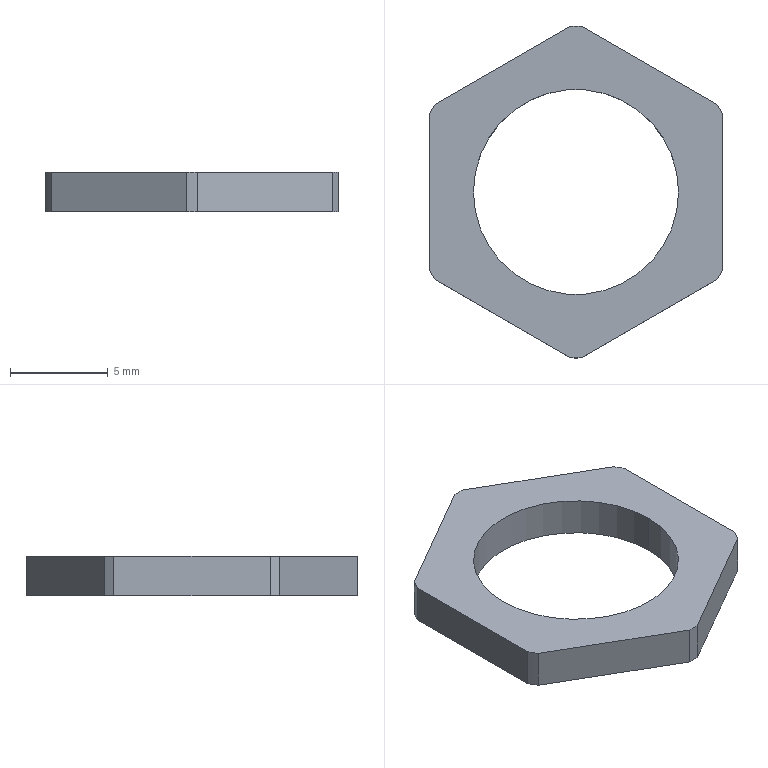Part | STEP file | 1 solid | 16 faces | box 15 x 17 x 2 mm | volume 215.987 mm3 | cylinder 8 | plane 8 | commonest cylinder face diameters 17 x6 10.5 x2
STEP:
#1=CARTESIAN_POINT('',(0.,0.,0.));
#2=DIRECTION('',(0.,0.,1.));
#3=DIRECTION('',(1.,0.,0.));
#4=AXIS2_PLACEMENT_3D('',#1,#2,#3);
#5=CARTESIAN_POINT('',(0.2859,8.495,2.));
#6=VERTEX_POINT('',#5);
#7=CARTESIAN_POINT('',(0.2859,8.495,0.));
#8=VERTEX_POINT('',#7);
#9=CARTESIAN_POINT('',(0.2859,8.495,0.));
#10=DIRECTION('',(0.,0.,-1.));
#11=VECTOR('',#10,1.);
#12=LINE('',#9,#11);
#13=CARTESIAN_POINT('',(0.,0.,0.));
#14=DIRECTION('',(0.,0.,1.));
#15=DIRECTION('',(1.,0.,0.));
#16=AXIS2_PLACEMENT_3D('',#13,#14,#15);
#17=CYLINDRICAL_SURFACE('',#16,8.5);
#18=CARTESIAN_POINT('',(1.537,0.));
#19=DIRECTION('',(0.,-1.));
#20=VECTOR('',#19,1.);
#21=LINE('',#18,#20);
#22=(GEOMETRIC_REPRESENTATION_CONTEXT(2)PARAMETRIC_REPRESENTATION_CONTEXT()REPRESENTATION_CONTEXT('',''));
#23=DEFINITIONAL_REPRESENTATION('',(#21),#22);
#24=PCURVE('',#17,#23);
#25=CARTESIAN_POINT('',(7.5,4.33,2.));
#26=DIRECTION('',(-0.5,-0.866,0.));
#27=DIRECTION('',(0.866,-0.5,0.));
#28=AXIS2_PLACEMENT_3D('',#25,#26,#27);
#29=PLANE('',#28);
#30=CARTESIAN_POINT('',(-8.33,-2.));
#31=DIRECTION('',(0.,-1.));
#32=VECTOR('',#31,1.);
#33=LINE('',#30,#32);
#34=(GEOMETRIC_REPRESENTATION_CONTEXT(2)PARAMETRIC_REPRESENTATION_CONTEXT()REPRESENTATION_CONTEXT('',''));
#35=DEFINITIONAL_REPRESENTATION('',(#33),#34);
#36=PCURVE('',#29,#35);
#37=SURFACE_CURVE('',#12,(#24,#36),.PCURVE_S1.);
#38=EDGE_CURVE('',#6,#8,#37,.T.);
#39=ORIENTED_EDGE('',*,*,#38,.T.);
#40=CARTESIAN_POINT('',(-0.2859,8.495,0.));
#41=VERTEX_POINT('',#40);
#42=CARTESIAN_POINT('',(0.,0.,0.));
#43=DIRECTION('',(0.,0.,1.));
#44=DIRECTION('',(1.,0.,0.));
#45=AXIS2_PLACEMENT_3D('',#42,#43,#44);
#46=CIRCLE('',#45,8.5);
#47=CARTESIAN_POINT('',(0.,0.));
#48=DIRECTION('',(1.,0.));
#49=VECTOR('',#48,1.);
#50=LINE('',#47,#49);
#51=(GEOMETRIC_REPRESENTATION_CONTEXT(2)PARAMETRIC_REPRESENTATION_CONTEXT()REPRESENTATION_CONTEXT('',''));
#52=DEFINITIONAL_REPRESENTATION('',(#50),#51);
#53=PCURVE('',#17,#52);
#54=CARTESIAN_POINT('',(0.,0.,0.));
#55=DIRECTION('',(0.,0.,1.));
#56=DIRECTION('',(1.,0.,0.));
#57=AXIS2_PLACEMENT_3D('',#54,#55,#56);
#58=PLANE('',#57);
#59=CARTESIAN_POINT('',(0.,0.));
#60=DIRECTION('',(1.,0.));
#61=AXIS2_PLACEMENT_2D('',#59,#60);
#62=CIRCLE('',#61,8.5);
#63=(GEOMETRIC_REPRESENTATION_CONTEXT(2)PARAMETRIC_REPRESENTATION_CONTEXT()REPRESENTATION_CONTEXT('',''));
#64=DEFINITIONAL_REPRESENTATION('',(#62),#63);
#65=PCURVE('',#58,#64);
#66=SURFACE_CURVE('',#46,(#53,#65),.PCURVE_S1.);
#67=EDGE_CURVE('',#8,#41,#66,.T.);
#68=ORIENTED_EDGE('',*,*,#67,.T.);
#69=CARTESIAN_POINT('',(-0.2859,8.495,2.));
#70=VERTEX_POINT('',#69);
#71=CARTESIAN_POINT('',(-0.2859,8.495,0.));
#72=DIRECTION('',(0.,0.,1.));
#73=VECTOR('',#72,1.);
#74=LINE('',#71,#73);
#75=CARTESIAN_POINT('',(1.604,0.));
#76=DIRECTION('',(0.,1.));
#77=VECTOR('',#76,1.);
#78=LINE('',#75,#77);
#79=(GEOMETRIC_REPRESENTATION_CONTEXT(2)PARAMETRIC_REPRESENTATION_CONTEXT()REPRESENTATION_CONTEXT('',''));
#80=DEFINITIONAL_REPRESENTATION('',(#78),#79);
#81=PCURVE('',#17,#80);
#82=CARTESIAN_POINT('',(0.,8.66,2.));
#83=DIRECTION('',(0.5,-0.866,0.));
#84=DIRECTION('',(0.866,0.5,0.));
#85=AXIS2_PLACEMENT_3D('',#82,#83,#84);
#86=PLANE('',#85);
#87=CARTESIAN_POINT('',(-0.3301,-2.));
#88=DIRECTION('',(0.,1.));
#89=VECTOR('',#88,1.);
#90=LINE('',#87,#89);
#91=(GEOMETRIC_REPRESENTATION_CONTEXT(2)PARAMETRIC_REPRESENTATION_CONTEXT()REPRESENTATION_CONTEXT('',''));
#92=DEFINITIONAL_REPRESENTATION('',(#90),#91);
#93=PCURVE('',#86,#92);
#94=SURFACE_CURVE('',#74,(#81,#93),.PCURVE_S1.);
#95=EDGE_CURVE('',#41,#70,#94,.T.);
#96=ORIENTED_EDGE('',*,*,#95,.T.);
#97=CARTESIAN_POINT('',(0.,0.,2.));
#98=DIRECTION('',(0.,0.,1.));
#99=DIRECTION('',(1.,0.,0.));
#100=AXIS2_PLACEMENT_3D('',#97,#98,#99);
#101=CIRCLE('',#100,8.5);
#102=CARTESIAN_POINT('',(0.,2.));
#103=DIRECTION('',(1.,0.));
#104=VECTOR('',#103,1.);
#105=LINE('',#102,#104);
#106=(GEOMETRIC_REPRESENTATION_CONTEXT(2)PARAMETRIC_REPRESENTATION_CONTEXT()REPRESENTATION_CONTEXT('',''));
#107=DEFINITIONAL_REPRESENTATION('',(#105),#106);
#108=PCURVE('',#17,#107);
#109=CARTESIAN_POINT('',(0.,0.,2.));
#110=DIRECTION('',(0.,0.,1.));
#111=DIRECTION('',(1.,0.,0.));
#112=AXIS2_PLACEMENT_3D('',#109,#110,#111);
#113=PLANE('',#112);
#114=CARTESIAN_POINT('',(0.,0.));
#115=DIRECTION('',(1.,0.));
#116=AXIS2_PLACEMENT_2D('',#114,#115);
#117=CIRCLE('',#116,8.5);
#118=(GEOMETRIC_REPRESENTATION_CONTEXT(2)PARAMETRIC_REPRESENTATION_CONTEXT()REPRESENTATION_CONTEXT('',''));
#119=DEFINITIONAL_REPRESENTATION('',(#117),#118);
#120=PCURVE('',#113,#119);
#121=SURFACE_CURVE('',#101,(#108,#120),.PCURVE_S1.);
#122=EDGE_CURVE('',#6,#70,#121,.T.);
#123=ORIENTED_EDGE('',*,*,#122,.F.);
#124=EDGE_LOOP('',(#39,#68,#96,#123));
#125=FACE_BOUND('',#124,.T.);
#126=ADVANCED_FACE('',(#125),#17,.T.);
#127=CARTESIAN_POINT('',(-7.214,4.495,2.));
#128=VERTEX_POINT('',#127);
#129=CARTESIAN_POINT('',(-7.214,4.495,0.));
#130=VERTEX_POINT('',#129);
#131=CARTESIAN_POINT('',(-7.214,4.495,0.));
#132=DIRECTION('',(0.,0.,-1.));
#133=VECTOR('',#132,1.);
#134=LINE('',#131,#133);
#135=CARTESIAN_POINT('',(0.,0.,0.));
#136=DIRECTION('',(0.,0.,1.));
#137=DIRECTION('',(1.,0.,0.));
#138=AXIS2_PLACEMENT_3D('',#135,#136,#137);
#139=CYLINDRICAL_SURFACE('',#138,8.5);
#140=CARTESIAN_POINT('',(2.584,0.));
#141=DIRECTION('',(0.,-1.));
#142=VECTOR('',#141,1.);
#143=LINE('',#140,#142);
#144=(GEOMETRIC_REPRESENTATION_CONTEXT(2)PARAMETRIC_REPRESENTATION_CONTEXT()REPRESENTATION_CONTEXT('',''));
#145=DEFINITIONAL_REPRESENTATION('',(#143),#144);
#146=PCURVE('',#139,#145);
#147=CARTESIAN_POINT('',(-8.33,-2.));
#148=DIRECTION('',(0.,-1.));
#149=VECTOR('',#148,1.);
#150=LINE('',#147,#149);
#151=(GEOMETRIC_REPRESENTATION_CONTEXT(2)PARAMETRIC_REPRESENTATION_CONTEXT()REPRESENTATION_CONTEXT('',''));
#152=DEFINITIONAL_REPRESENTATION('',(#150),#151);
#153=PCURVE('',#86,#152);
#154=SURFACE_CURVE('',#134,(#146,#153),.PCURVE_S1.);
#155=EDGE_CURVE('',#128,#130,#154,.T.);
#156=ORIENTED_EDGE('',*,*,#155,.T.);
#157=CARTESIAN_POINT('',(-7.5,4.,0.));
#158=VERTEX_POINT('',#157);
#159=CARTESIAN_POINT('',(0.,0.,0.));
#160=DIRECTION('',(0.,0.,1.));
#161=DIRECTION('',(1.,0.,0.));
#162=AXIS2_PLACEMENT_3D('',#159,#160,#161);
#163=CIRCLE('',#162,8.5);
#164=CARTESIAN_POINT('',(0.,0.));
#165=DIRECTION('',(1.,0.));
#166=VECTOR('',#165,1.);
#167=LINE('',#164,#166);
#168=(GEOMETRIC_REPRESENTATION_CONTEXT(2)PARAMETRIC_REPRESENTATION_CONTEXT()REPRESENTATION_CONTEXT('',''));
#169=DEFINITIONAL_REPRESENTATION('',(#167),#168);
#170=PCURVE('',#139,#169);
#171=CARTESIAN_POINT('',(0.,0.));
#172=DIRECTION('',(1.,0.));
#173=AXIS2_PLACEMENT_2D('',#171,#172);
#174=CIRCLE('',#173,8.5);
#175=(GEOMETRIC_REPRESENTATION_CONTEXT(2)PARAMETRIC_REPRESENTATION_CONTEXT()REPRESENTATION_CONTEXT('',''));
#176=DEFINITIONAL_REPRESENTATION('',(#174),#175);
#177=PCURVE('',#58,#176);
#178=SURFACE_CURVE('',#163,(#170,#177),.PCURVE_S1.);
#179=EDGE_CURVE('',#130,#158,#178,.T.);
#180=ORIENTED_EDGE('',*,*,#179,.T.);
#181=CARTESIAN_POINT('',(-7.5,4.,2.));
#182=VERTEX_POINT('',#181);
#183=CARTESIAN_POINT('',(-7.5,4.,0.));
#184=DIRECTION('',(0.,0.,1.));
#185=VECTOR('',#184,1.);
#186=LINE('',#183,#185);
#187=CARTESIAN_POINT('',(2.652,0.));
#188=DIRECTION('',(0.,1.));
#189=VECTOR('',#188,1.);
#190=LINE('',#187,#189);
#191=(GEOMETRIC_REPRESENTATION_CONTEXT(2)PARAMETRIC_REPRESENTATION_CONTEXT()REPRESENTATION_CONTEXT('',''));
#192=DEFINITIONAL_REPRESENTATION('',(#190),#191);
#193=PCURVE('',#139,#192);
#194=CARTESIAN_POINT('',(-7.5,4.33,2.));
#195=DIRECTION('',(1.,0.,0.));
#196=DIRECTION('',(0.,1.,0.));
#197=AXIS2_PLACEMENT_3D('',#194,#195,#196);
#198=PLANE('',#197);
#199=CARTESIAN_POINT('',(-0.3301,-2.));
#200=DIRECTION('',(0.,1.));
#201=VECTOR('',#200,1.);
#202=LINE('',#199,#201);
#203=(GEOMETRIC_REPRESENTATION_CONTEXT(2)PARAMETRIC_REPRESENTATION_CONTEXT()REPRESENTATION_CONTEXT('',''));
#204=DEFINITIONAL_REPRESENTATION('',(#202),#203);
#205=PCURVE('',#198,#204);
#206=SURFACE_CURVE('',#186,(#193,#205),.PCURVE_S1.);
#207=EDGE_CURVE('',#158,#182,#206,.T.);
#208=ORIENTED_EDGE('',*,*,#207,.T.);
#209=CARTESIAN_POINT('',(0.,0.,2.));
#210=DIRECTION('',(0.,0.,1.));
#211=DIRECTION('',(1.,0.,0.));
#212=AXIS2_PLACEMENT_3D('',#209,#210,#211);
#213=CIRCLE('',#212,8.5);
#214=CARTESIAN_POINT('',(0.,2.));
#215=DIRECTION('',(1.,0.));
#216=VECTOR('',#215,1.);
#217=LINE('',#214,#216);
#218=(GEOMETRIC_REPRESENTATION_CONTEXT(2)PARAMETRIC_REPRESENTATION_CONTEXT()REPRESENTATION_CONTEXT('',''));
#219=DEFINITIONAL_REPRESENTATION('',(#217),#218);
#220=PCURVE('',#139,#219);
#221=CARTESIAN_POINT('',(0.,0.));
#222=DIRECTION('',(1.,0.));
#223=AXIS2_PLACEMENT_2D('',#221,#222);
#224=CIRCLE('',#223,8.5);
#225=(GEOMETRIC_REPRESENTATION_CONTEXT(2)PARAMETRIC_REPRESENTATION_CONTEXT()REPRESENTATION_CONTEXT('',''));
#226=DEFINITIONAL_REPRESENTATION('',(#224),#225);
#227=PCURVE('',#113,#226);
#228=SURFACE_CURVE('',#213,(#220,#227),.PCURVE_S1.);
#229=EDGE_CURVE('',#128,#182,#228,.T.);
#230=ORIENTED_EDGE('',*,*,#229,.F.);
#231=EDGE_LOOP('',(#156,#180,#208,#230));
#232=FACE_BOUND('',#231,.T.);
#233=ADVANCED_FACE('',(#232),#139,.T.);
#234=CARTESIAN_POINT('',(-7.5,-4.,2.));
#235=VERTEX_POINT('',#234);
#236=CARTESIAN_POINT('',(-7.5,-4.,0.));
#237=VERTEX_POINT('',#236);
#238=CARTESIAN_POINT('',(-7.5,-4.,0.));
#239=DIRECTION('',(0.,0.,-1.));
#240=VECTOR('',#239,1.);
#241=LINE('',#238,#240);
#242=CARTESIAN_POINT('',(0.,0.,0.));
#243=DIRECTION('',(0.,0.,1.));
#244=DIRECTION('',(1.,0.,0.));
#245=AXIS2_PLACEMENT_3D('',#242,#243,#244);
#246=CYLINDRICAL_SURFACE('',#245,8.5);
#247=CARTESIAN_POINT('',(3.632,0.));
#248=DIRECTION('',(0.,-1.));
#249=VECTOR('',#248,1.);
#250=LINE('',#247,#249);
#251=(GEOMETRIC_REPRESENTATION_CONTEXT(2)PARAMETRIC_REPRESENTATION_CONTEXT()REPRESENTATION_CONTEXT('',''));
#252=DEFINITIONAL_REPRESENTATION('',(#250),#251);
#253=PCURVE('',#246,#252);
#254=CARTESIAN_POINT('',(-8.33,-2.));
#255=DIRECTION('',(0.,-1.));
#256=VECTOR('',#255,1.);
#257=LINE('',#254,#256);
#258=(GEOMETRIC_REPRESENTATION_CONTEXT(2)PARAMETRIC_REPRESENTATION_CONTEXT()REPRESENTATION_CONTEXT('',''));
#259=DEFINITIONAL_REPRESENTATION('',(#257),#258);
#260=PCURVE('',#198,#259);
#261=SURFACE_CURVE('',#241,(#253,#260),.PCURVE_S1.);
#262=EDGE_CURVE('',#235,#237,#261,.T.);
#263=ORIENTED_EDGE('',*,*,#262,.T.);
#264=CARTESIAN_POINT('',(-7.214,-4.495,0.));
#265=VERTEX_POINT('',#264);
#266=CARTESIAN_POINT('',(0.,0.,0.));
#267=DIRECTION('',(0.,0.,1.));
#268=DIRECTION('',(1.,0.,0.));
#269=AXIS2_PLACEMENT_3D('',#266,#267,#268);
#270=CIRCLE('',#269,8.5);
#271=CARTESIAN_POINT('',(0.,0.));
#272=DIRECTION('',(1.,0.));
#273=VECTOR('',#272,1.);
#274=LINE('',#271,#273);
#275=(GEOMETRIC_REPRESENTATION_CONTEXT(2)PARAMETRIC_REPRESENTATION_CONTEXT()REPRESENTATION_CONTEXT('',''));
#276=DEFINITIONAL_REPRESENTATION('',(#274),#275);
#277=PCURVE('',#246,#276);
#278=CARTESIAN_POINT('',(0.,0.));
#279=DIRECTION('',(1.,0.));
#280=AXIS2_PLACEMENT_2D('',#278,#279);
#281=CIRCLE('',#280,8.5);
#282=(GEOMETRIC_REPRESENTATION_CONTEXT(2)PARAMETRIC_REPRESENTATION_CONTEXT()REPRESENTATION_CONTEXT('',''));
#283=DEFINITIONAL_REPRESENTATION('',(#281),#282);
#284=PCURVE('',#58,#283);
#285=SURFACE_CURVE('',#270,(#277,#284),.PCURVE_S1.);
#286=EDGE_CURVE('',#237,#265,#285,.T.);
#287=ORIENTED_EDGE('',*,*,#286,.T.);
#288=CARTESIAN_POINT('',(-7.214,-4.495,2.));
#289=VERTEX_POINT('',#288);
#290=CARTESIAN_POINT('',(-7.214,-4.495,0.));
#291=DIRECTION('',(0.,0.,1.));
#292=VECTOR('',#291,1.);
#293=LINE('',#290,#292);
#294=CARTESIAN_POINT('',(3.699,0.));
#295=DIRECTION('',(0.,1.));
#296=VECTOR('',#295,1.);
#297=LINE('',#294,#296);
#298=(GEOMETRIC_REPRESENTATION_CONTEXT(2)PARAMETRIC_REPRESENTATION_CONTEXT()REPRESENTATION_CONTEXT('',''));
#299=DEFINITIONAL_REPRESENTATION('',(#297),#298);
#300=PCURVE('',#246,#299);
#301=CARTESIAN_POINT('',(-7.5,-4.33,2.));
#302=DIRECTION('',(0.5,0.866,0.));
#303=DIRECTION('',(-0.866,0.5,0.));
#304=AXIS2_PLACEMENT_3D('',#301,#302,#303);
#305=PLANE('',#304);
#306=CARTESIAN_POINT('',(-0.3301,-2.));
#307=DIRECTION('',(0.,1.));
#308=VECTOR('',#307,1.);
#309=LINE('',#306,#308);
#310=(GEOMETRIC_REPRESENTATION_CONTEXT(2)PARAMETRIC_REPRESENTATION_CONTEXT()REPRESENTATION_CONTEXT('',''));
#311=DEFINITIONAL_REPRESENTATION('',(#309),#310);
#312=PCURVE('',#305,#311);
#313=SURFACE_CURVE('',#293,(#300,#312),.PCURVE_S1.);
#314=EDGE_CURVE('',#265,#289,#313,.T.);
#315=ORIENTED_EDGE('',*,*,#314,.T.);
#316=CARTESIAN_POINT('',(0.,0.,2.));
#317=DIRECTION('',(0.,0.,1.));
#318=DIRECTION('',(1.,0.,0.));
#319=AXIS2_PLACEMENT_3D('',#316,#317,#318);
#320=CIRCLE('',#319,8.5);
#321=CARTESIAN_POINT('',(0.,2.));
#322=DIRECTION('',(1.,0.));
#323=VECTOR('',#322,1.);
#324=LINE('',#321,#323);
#325=(GEOMETRIC_REPRESENTATION_CONTEXT(2)PARAMETRIC_REPRESENTATION_CONTEXT()REPRESENTATION_CONTEXT('',''));
#326=DEFINITIONAL_REPRESENTATION('',(#324),#325);
#327=PCURVE('',#246,#326);
#328=CARTESIAN_POINT('',(0.,0.));
#329=DIRECTION('',(1.,0.));
#330=AXIS2_PLACEMENT_2D('',#328,#329);
#331=CIRCLE('',#330,8.5);
#332=(GEOMETRIC_REPRESENTATION_CONTEXT(2)PARAMETRIC_REPRESENTATION_CONTEXT()REPRESENTATION_CONTEXT('',''));
#333=DEFINITIONAL_REPRESENTATION('',(#331),#332);
#334=PCURVE('',#113,#333);
#335=SURFACE_CURVE('',#320,(#327,#334),.PCURVE_S1.);
#336=EDGE_CURVE('',#235,#289,#335,.T.);
#337=ORIENTED_EDGE('',*,*,#336,.F.);
#338=EDGE_LOOP('',(#263,#287,#315,#337));
#339=FACE_BOUND('',#338,.T.);
#340=ADVANCED_FACE('',(#339),#246,.T.);
#341=CARTESIAN_POINT('',(-0.2859,-8.495,2.));
#342=VERTEX_POINT('',#341);
#343=CARTESIAN_POINT('',(-0.2859,-8.495,0.));
#344=VERTEX_POINT('',#343);
#345=CARTESIAN_POINT('',(-0.2859,-8.495,0.));
#346=DIRECTION('',(0.,0.,-1.));
#347=VECTOR('',#346,1.);
#348=LINE('',#345,#347);
#349=CARTESIAN_POINT('',(0.,0.,0.));
#350=DIRECTION('',(0.,0.,1.));
#351=DIRECTION('',(1.,0.,0.));
#352=AXIS2_PLACEMENT_3D('',#349,#350,#351);
#353=CYLINDRICAL_SURFACE('',#352,8.5);
#354=CARTESIAN_POINT('',(4.679,0.));
#355=DIRECTION('',(0.,-1.));
#356=VECTOR('',#355,1.);
#357=LINE('',#354,#356);
#358=(GEOMETRIC_REPRESENTATION_CONTEXT(2)PARAMETRIC_REPRESENTATION_CONTEXT()REPRESENTATION_CONTEXT('',''));
#359=DEFINITIONAL_REPRESENTATION('',(#357),#358);
#360=PCURVE('',#353,#359);
#361=CARTESIAN_POINT('',(-8.33,-2.));
#362=DIRECTION('',(0.,-1.));
#363=VECTOR('',#362,1.);
#364=LINE('',#361,#363);
#365=(GEOMETRIC_REPRESENTATION_CONTEXT(2)PARAMETRIC_REPRESENTATION_CONTEXT()REPRESENTATION_CONTEXT('',''));
#366=DEFINITIONAL_REPRESENTATION('',(#364),#365);
#367=PCURVE('',#305,#366);
#368=SURFACE_CURVE('',#348,(#360,#367),.PCURVE_S1.);
#369=EDGE_CURVE('',#342,#344,#368,.T.);
#370=ORIENTED_EDGE('',*,*,#369,.T.);
#371=CARTESIAN_POINT('',(0.2859,-8.495,0.));
#372=VERTEX_POINT('',#371);
#373=CARTESIAN_POINT('',(0.,0.,0.));
#374=DIRECTION('',(0.,0.,1.));
#375=DIRECTION('',(1.,0.,0.));
#376=AXIS2_PLACEMENT_3D('',#373,#374,#375);
#377=CIRCLE('',#376,8.5);
#378=CARTESIAN_POINT('',(0.,0.));
#379=DIRECTION('',(1.,0.));
#380=VECTOR('',#379,1.);
#381=LINE('',#378,#380);
#382=(GEOMETRIC_REPRESENTATION_CONTEXT(2)PARAMETRIC_REPRESENTATION_CONTEXT()REPRESENTATION_CONTEXT('',''));
#383=DEFINITIONAL_REPRESENTATION('',(#381),#382);
#384=PCURVE('',#353,#383);
#385=CARTESIAN_POINT('',(0.,0.));
#386=DIRECTION('',(1.,0.));
#387=AXIS2_PLACEMENT_2D('',#385,#386);
#388=CIRCLE('',#387,8.5);
#389=(GEOMETRIC_REPRESENTATION_CONTEXT(2)PARAMETRIC_REPRESENTATION_CONTEXT()REPRESENTATION_CONTEXT('',''));
#390=DEFINITIONAL_REPRESENTATION('',(#388),#389);
#391=PCURVE('',#58,#390);
#392=SURFACE_CURVE('',#377,(#384,#391),.PCURVE_S1.);
#393=EDGE_CURVE('',#344,#372,#392,.T.);
#394=ORIENTED_EDGE('',*,*,#393,.T.);
#395=CARTESIAN_POINT('',(0.2859,-8.495,2.));
#396=VERTEX_POINT('',#395);
#397=CARTESIAN_POINT('',(0.2859,-8.495,0.));
#398=DIRECTION('',(0.,0.,1.));
#399=VECTOR('',#398,1.);
#400=LINE('',#397,#399);
#401=CARTESIAN_POINT('',(4.746,0.));
#402=DIRECTION('',(0.,1.));
#403=VECTOR('',#402,1.);
#404=LINE('',#401,#403);
#405=(GEOMETRIC_REPRESENTATION_CONTEXT(2)PARAMETRIC_REPRESENTATION_CONTEXT()REPRESENTATION_CONTEXT('',''));
#406=DEFINITIONAL_REPRESENTATION('',(#404),#405);
#407=PCURVE('',#353,#406);
#408=CARTESIAN_POINT('',(0.,-8.66,2.));
#409=DIRECTION('',(-0.5,0.866,0.));
#410=DIRECTION('',(-0.866,-0.5,0.));
#411=AXIS2_PLACEMENT_3D('',#408,#409,#410);
#412=PLANE('',#411);
#413=CARTESIAN_POINT('',(-0.3301,-2.));
#414=DIRECTION('',(0.,1.));
#415=VECTOR('',#414,1.);
#416=LINE('',#413,#415);
#417=(GEOMETRIC_REPRESENTATION_CONTEXT(2)PARAMETRIC_REPRESENTATION_CONTEXT()REPRESENTATION_CONTEXT('',''));
#418=DEFINITIONAL_REPRESENTATION('',(#416),#417);
#419=PCURVE('',#412,#418);
#420=SURFACE_CURVE('',#400,(#407,#419),.PCURVE_S1.);
#421=EDGE_CURVE('',#372,#396,#420,.T.);
#422=ORIENTED_EDGE('',*,*,#421,.T.);
#423=CARTESIAN_POINT('',(0.,0.,2.));
#424=DIRECTION('',(0.,0.,1.));
#425=DIRECTION('',(1.,0.,0.));
#426=AXIS2_PLACEMENT_3D('',#423,#424,#425);
#427=CIRCLE('',#426,8.5);
#428=CARTESIAN_POINT('',(0.,2.));
#429=DIRECTION('',(1.,0.));
#430=VECTOR('',#429,1.);
#431=LINE('',#428,#430);
#432=(GEOMETRIC_REPRESENTATION_CONTEXT(2)PARAMETRIC_REPRESENTATION_CONTEXT()REPRESENTATION_CONTEXT('',''));
#433=DEFINITIONAL_REPRESENTATION('',(#431),#432);
#434=PCURVE('',#353,#433);
#435=CARTESIAN_POINT('',(0.,0.));
#436=DIRECTION('',(1.,0.));
#437=AXIS2_PLACEMENT_2D('',#435,#436);
#438=CIRCLE('',#437,8.5);
#439=(GEOMETRIC_REPRESENTATION_CONTEXT(2)PARAMETRIC_REPRESENTATION_CONTEXT()REPRESENTATION_CONTEXT('',''));
#440=DEFINITIONAL_REPRESENTATION('',(#438),#439);
#441=PCURVE('',#113,#440);
#442=SURFACE_CURVE('',#427,(#434,#441),.PCURVE_S1.);
#443=EDGE_CURVE('',#342,#396,#442,.T.);
#444=ORIENTED_EDGE('',*,*,#443,.F.);
#445=EDGE_LOOP('',(#370,#394,#422,#444));
#446=FACE_BOUND('',#445,.T.);
#447=ADVANCED_FACE('',(#446),#353,.T.);
#448=CARTESIAN_POINT('',(7.214,-4.495,2.));
#449=VERTEX_POINT('',#448);
#450=CARTESIAN_POINT('',(7.214,-4.495,0.));
#451=VERTEX_POINT('',#450);
#452=CARTESIAN_POINT('',(7.214,-4.495,0.));
#453=DIRECTION('',(0.,0.,-1.));
#454=VECTOR('',#453,1.);
#455=LINE('',#452,#454);
#456=CARTESIAN_POINT('',(0.,0.,0.));
#457=DIRECTION('',(0.,0.,1.));
#458=DIRECTION('',(1.,0.,0.));
#459=AXIS2_PLACEMENT_3D('',#456,#457,#458);
#460=CYLINDRICAL_SURFACE('',#459,8.5);
#461=CARTESIAN_POINT('',(5.726,0.));
#462=DIRECTION('',(0.,-1.));
#463=VECTOR('',#462,1.);
#464=LINE('',#461,#463);
#465=(GEOMETRIC_REPRESENTATION_CONTEXT(2)PARAMETRIC_REPRESENTATION_CONTEXT()REPRESENTATION_CONTEXT('',''));
#466=DEFINITIONAL_REPRESENTATION('',(#464),#465);
#467=PCURVE('',#460,#466);
#468=CARTESIAN_POINT('',(-8.33,-2.));
#469=DIRECTION('',(0.,-1.));
#470=VECTOR('',#469,1.);
#471=LINE('',#468,#470);
#472=(GEOMETRIC_REPRESENTATION_CONTEXT(2)PARAMETRIC_REPRESENTATION_CONTEXT()REPRESENTATION_CONTEXT('',''));
#473=DEFINITIONAL_REPRESENTATION('',(#471),#472);
#474=PCURVE('',#412,#473);
#475=SURFACE_CURVE('',#455,(#467,#474),.PCURVE_S1.);
#476=EDGE_CURVE('',#449,#451,#475,.T.);
#477=ORIENTED_EDGE('',*,*,#476,.T.);
#478=CARTESIAN_POINT('',(7.5,-4.,0.));
#479=VERTEX_POINT('',#478);
#480=CARTESIAN_POINT('',(0.,0.,0.));
#481=DIRECTION('',(0.,0.,1.));
#482=DIRECTION('',(1.,0.,0.));
#483=AXIS2_PLACEMENT_3D('',#480,#481,#482);
#484=CIRCLE('',#483,8.5);
#485=CARTESIAN_POINT('',(0.,0.));
#486=DIRECTION('',(1.,0.));
#487=VECTOR('',#486,1.);
#488=LINE('',#485,#487);
#489=(GEOMETRIC_REPRESENTATION_CONTEXT(2)PARAMETRIC_REPRESENTATION_CONTEXT()REPRESENTATION_CONTEXT('',''));
#490=DEFINITIONAL_REPRESENTATION('',(#488),#489);
#491=PCURVE('',#460,#490);
#492=CARTESIAN_POINT('',(0.,0.));
#493=DIRECTION('',(1.,0.));
#494=AXIS2_PLACEMENT_2D('',#492,#493);
#495=CIRCLE('',#494,8.5);
#496=(GEOMETRIC_REPRESENTATION_CONTEXT(2)PARAMETRIC_REPRESENTATION_CONTEXT()REPRESENTATION_CONTEXT('',''));
#497=DEFINITIONAL_REPRESENTATION('',(#495),#496);
#498=PCURVE('',#58,#497);
#499=SURFACE_CURVE('',#484,(#491,#498),.PCURVE_S1.);
#500=EDGE_CURVE('',#451,#479,#499,.T.);
#501=ORIENTED_EDGE('',*,*,#500,.T.);
#502=CARTESIAN_POINT('',(7.5,-4.,2.));
#503=VERTEX_POINT('',#502);
#504=CARTESIAN_POINT('',(7.5,-4.,0.));
#505=DIRECTION('',(0.,0.,1.));
#506=VECTOR('',#505,1.);
#507=LINE('',#504,#506);
#508=CARTESIAN_POINT('',(5.793,0.));
#509=DIRECTION('',(0.,1.));
#510=VECTOR('',#509,1.);
#511=LINE('',#508,#510);
#512=(GEOMETRIC_REPRESENTATION_CONTEXT(2)PARAMETRIC_REPRESENTATION_CONTEXT()REPRESENTATION_CONTEXT('',''));
#513=DEFINITIONAL_REPRESENTATION('',(#511),#512);
#514=PCURVE('',#460,#513);
#515=CARTESIAN_POINT('',(7.5,-4.33,2.));
#516=DIRECTION('',(-1.,0.,0.));
#517=DIRECTION('',(0.,-1.,0.));
#518=AXIS2_PLACEMENT_3D('',#515,#516,#517);
#519=PLANE('',#518);
#520=CARTESIAN_POINT('',(-0.3301,-2.));
#521=DIRECTION('',(0.,1.));
#522=VECTOR('',#521,1.);
#523=LINE('',#520,#522);
#524=(GEOMETRIC_REPRESENTATION_CONTEXT(2)PARAMETRIC_REPRESENTATION_CONTEXT()REPRESENTATION_CONTEXT('',''));
#525=DEFINITIONAL_REPRESENTATION('',(#523),#524);
#526=PCURVE('',#519,#525);
#527=SURFACE_CURVE('',#507,(#514,#526),.PCURVE_S1.);
#528=EDGE_CURVE('',#479,#503,#527,.T.);
#529=ORIENTED_EDGE('',*,*,#528,.T.);
#530=CARTESIAN_POINT('',(0.,0.,2.));
#531=DIRECTION('',(0.,0.,1.));
#532=DIRECTION('',(1.,0.,0.));
#533=AXIS2_PLACEMENT_3D('',#530,#531,#532);
#534=CIRCLE('',#533,8.5);
#535=CARTESIAN_POINT('',(0.,2.));
#536=DIRECTION('',(1.,0.));
#537=VECTOR('',#536,1.);
#538=LINE('',#535,#537);
#539=(GEOMETRIC_REPRESENTATION_CONTEXT(2)PARAMETRIC_REPRESENTATION_CONTEXT()REPRESENTATION_CONTEXT('',''));
#540=DEFINITIONAL_REPRESENTATION('',(#538),#539);
#541=PCURVE('',#460,#540);
#542=CARTESIAN_POINT('',(0.,0.));
#543=DIRECTION('',(1.,0.));
#544=AXIS2_PLACEMENT_2D('',#542,#543);
#545=CIRCLE('',#544,8.5);
#546=(GEOMETRIC_REPRESENTATION_CONTEXT(2)PARAMETRIC_REPRESENTATION_CONTEXT()REPRESENTATION_CONTEXT('',''));
#547=DEFINITIONAL_REPRESENTATION('',(#545),#546);
#548=PCURVE('',#113,#547);
#549=SURFACE_CURVE('',#534,(#541,#548),.PCURVE_S1.);
#550=EDGE_CURVE('',#449,#503,#549,.T.);
#551=ORIENTED_EDGE('',*,*,#550,.F.);
#552=EDGE_LOOP('',(#477,#501,#529,#551));
#553=FACE_BOUND('',#552,.T.);
#554=ADVANCED_FACE('',(#553),#460,.T.);
#555=CARTESIAN_POINT('',(7.214,4.495,0.));
#556=VERTEX_POINT('',#555);
#557=CARTESIAN_POINT('',(7.214,4.495,2.));
#558=VERTEX_POINT('',#557);
#559=CARTESIAN_POINT('',(7.214,4.495,0.));
#560=DIRECTION('',(0.,0.,1.));
#561=VECTOR('',#560,1.);
#562=LINE('',#559,#561);
#563=CARTESIAN_POINT('',(0.,0.,0.));
#564=DIRECTION('',(0.,0.,1.));
#565=DIRECTION('',(1.,0.,0.));
#566=AXIS2_PLACEMENT_3D('',#563,#564,#565);
#567=CYLINDRICAL_SURFACE('',#566,8.5);
#568=CARTESIAN_POINT('',(0.5572,0.));
#569=DIRECTION('',(0.,1.));
#570=VECTOR('',#569,1.);
#571=LINE('',#568,#570);
#572=(GEOMETRIC_REPRESENTATION_CONTEXT(2)PARAMETRIC_REPRESENTATION_CONTEXT()REPRESENTATION_CONTEXT('',''));
#573=DEFINITIONAL_REPRESENTATION('',(#571),#572);
#574=PCURVE('',#567,#573);
#575=CARTESIAN_POINT('',(-0.3301,-2.));
#576=DIRECTION('',(0.,1.));
#577=VECTOR('',#576,1.);
#578=LINE('',#575,#577);
#579=(GEOMETRIC_REPRESENTATION_CONTEXT(2)PARAMETRIC_REPRESENTATION_CONTEXT()REPRESENTATION_CONTEXT('',''));
#580=DEFINITIONAL_REPRESENTATION('',(#578),#579);
#581=PCURVE('',#29,#580);
#582=SURFACE_CURVE('',#562,(#574,#581),.PCURVE_S1.);
#583=EDGE_CURVE('',#556,#558,#582,.T.);
#584=ORIENTED_EDGE('',*,*,#583,.T.);
#585=CARTESIAN_POINT('',(7.5,4.,2.));
#586=VERTEX_POINT('',#585);
#587=CARTESIAN_POINT('',(0.,0.,2.));
#588=DIRECTION('',(0.,0.,1.));
#589=DIRECTION('',(1.,0.,0.));
#590=AXIS2_PLACEMENT_3D('',#587,#588,#589);
#591=CIRCLE('',#590,8.5);
#592=CARTESIAN_POINT('',(0.,2.));
#593=DIRECTION('',(1.,0.));
#594=VECTOR('',#593,1.);
#595=LINE('',#592,#594);
#596=(GEOMETRIC_REPRESENTATION_CONTEXT(2)PARAMETRIC_REPRESENTATION_CONTEXT()REPRESENTATION_CONTEXT('',''));
#597=DEFINITIONAL_REPRESENTATION('',(#595),#596);
#598=PCURVE('',#567,#597);
#599=CARTESIAN_POINT('',(0.,0.));
#600=DIRECTION('',(1.,0.));
#601=AXIS2_PLACEMENT_2D('',#599,#600);
#602=CIRCLE('',#601,8.5);
#603=(GEOMETRIC_REPRESENTATION_CONTEXT(2)PARAMETRIC_REPRESENTATION_CONTEXT()REPRESENTATION_CONTEXT('',''));
#604=DEFINITIONAL_REPRESENTATION('',(#602),#603);
#605=PCURVE('',#113,#604);
#606=SURFACE_CURVE('',#591,(#598,#605),.PCURVE_S1.);
#607=EDGE_CURVE('',#586,#558,#606,.T.);
#608=ORIENTED_EDGE('',*,*,#607,.F.);
#609=CARTESIAN_POINT('',(7.5,4.,0.));
#610=VERTEX_POINT('',#609);
#611=CARTESIAN_POINT('',(7.5,4.,0.));
#612=DIRECTION('',(0.,0.,-1.));
#613=VECTOR('',#612,1.);
#614=LINE('',#611,#613);
#615=CARTESIAN_POINT('',(0.49,0.));
#616=DIRECTION('',(0.,-1.));
#617=VECTOR('',#616,1.);
#618=LINE('',#615,#617);
#619=(GEOMETRIC_REPRESENTATION_CONTEXT(2)PARAMETRIC_REPRESENTATION_CONTEXT()REPRESENTATION_CONTEXT('',''));
#620=DEFINITIONAL_REPRESENTATION('',(#618),#619);
#621=PCURVE('',#567,#620);
#622=CARTESIAN_POINT('',(-8.33,-2.));
#623=DIRECTION('',(0.,-1.));
#624=VECTOR('',#623,1.);
#625=LINE('',#622,#624);
#626=(GEOMETRIC_REPRESENTATION_CONTEXT(2)PARAMETRIC_REPRESENTATION_CONTEXT()REPRESENTATION_CONTEXT('',''));
#627=DEFINITIONAL_REPRESENTATION('',(#625),#626);
#628=PCURVE('',#519,#627);
#629=SURFACE_CURVE('',#614,(#621,#628),.PCURVE_S1.);
#630=EDGE_CURVE('',#586,#610,#629,.T.);
#631=ORIENTED_EDGE('',*,*,#630,.T.);
#632=CARTESIAN_POINT('',(0.,0.,0.));
#633=DIRECTION('',(0.,0.,1.));
#634=DIRECTION('',(1.,0.,0.));
#635=AXIS2_PLACEMENT_3D('',#632,#633,#634);
#636=CIRCLE('',#635,8.5);
#637=CARTESIAN_POINT('',(0.,0.));
#638=DIRECTION('',(1.,0.));
#639=VECTOR('',#638,1.);
#640=LINE('',#637,#639);
#641=(GEOMETRIC_REPRESENTATION_CONTEXT(2)PARAMETRIC_REPRESENTATION_CONTEXT()REPRESENTATION_CONTEXT('',''));
#642=DEFINITIONAL_REPRESENTATION('',(#640),#641);
#643=PCURVE('',#567,#642);
#644=CARTESIAN_POINT('',(0.,0.));
#645=DIRECTION('',(1.,0.));
#646=AXIS2_PLACEMENT_2D('',#644,#645);
#647=CIRCLE('',#646,8.5);
#648=(GEOMETRIC_REPRESENTATION_CONTEXT(2)PARAMETRIC_REPRESENTATION_CONTEXT()REPRESENTATION_CONTEXT('',''));
#649=DEFINITIONAL_REPRESENTATION('',(#647),#648);
#650=PCURVE('',#58,#649);
#651=SURFACE_CURVE('',#636,(#643,#650),.PCURVE_S1.);
#652=EDGE_CURVE('',#610,#556,#651,.T.);
#653=ORIENTED_EDGE('',*,*,#652,.T.);
#654=EDGE_LOOP('',(#584,#608,#631,#653));
#655=FACE_BOUND('',#654,.T.);
#656=ADVANCED_FACE('',(#655),#567,.T.);
#657=CARTESIAN_POINT('',(5.25,0.,2.));
#658=VERTEX_POINT('',#657);
#659=CARTESIAN_POINT('',(-5.25,0.,2.));
#660=VERTEX_POINT('',#659);
#661=CARTESIAN_POINT('',(0.,0.,2.));
#662=DIRECTION('',(0.,0.,1.));
#663=DIRECTION('',(1.,0.,0.));
#664=AXIS2_PLACEMENT_3D('',#661,#662,#663);
#665=CIRCLE('',#664,5.25);
#666=CARTESIAN_POINT('',(0.,0.,2.));
#667=DIRECTION('',(0.,0.,1.));
#668=DIRECTION('',(1.,0.,0.));
#669=AXIS2_PLACEMENT_3D('',#666,#667,#668);
#670=CYLINDRICAL_SURFACE('',#669,5.25);
#671=CARTESIAN_POINT('',(0.,0.));
#672=DIRECTION('',(1.,0.));
#673=VECTOR('',#672,1.);
#674=LINE('',#671,#673);
#675=(GEOMETRIC_REPRESENTATION_CONTEXT(2)PARAMETRIC_REPRESENTATION_CONTEXT()REPRESENTATION_CONTEXT('',''));
#676=DEFINITIONAL_REPRESENTATION('',(#674),#675);
#677=PCURVE('',#670,#676);
#678=CARTESIAN_POINT('',(0.,0.));
#679=DIRECTION('',(1.,0.));
#680=AXIS2_PLACEMENT_2D('',#678,#679);
#681=CIRCLE('',#680,5.25);
#682=(GEOMETRIC_REPRESENTATION_CONTEXT(2)PARAMETRIC_REPRESENTATION_CONTEXT()REPRESENTATION_CONTEXT('',''));
#683=DEFINITIONAL_REPRESENTATION('',(#681),#682);
#684=PCURVE('',#113,#683);
#685=SURFACE_CURVE('',#665,(#677,#684),.PCURVE_S1.);
#686=EDGE_CURVE('',#658,#660,#685,.T.);
#687=ORIENTED_EDGE('',*,*,#686,.F.);
#688=CARTESIAN_POINT('',(5.25,0.,0.));
#689=VERTEX_POINT('',#688);
#690=CARTESIAN_POINT('',(5.25,0.,2.));
#691=DIRECTION('',(0.,0.,1.));
#692=VECTOR('',#691,1.);
#693=LINE('',#690,#692);
#694=CARTESIAN_POINT('',(0.,0.));
#695=DIRECTION('',(0.,1.));
#696=VECTOR('',#695,1.);
#697=LINE('',#694,#696);
#698=(GEOMETRIC_REPRESENTATION_CONTEXT(2)PARAMETRIC_REPRESENTATION_CONTEXT()REPRESENTATION_CONTEXT('',''));
#699=DEFINITIONAL_REPRESENTATION('',(#697),#698);
#700=PCURVE('',#670,#699);
#701=CARTESIAN_POINT('',(0.,0.,2.));
#702=DIRECTION('',(0.,0.,1.));
#703=DIRECTION('',(1.,0.,0.));
#704=AXIS2_PLACEMENT_3D('',#701,#702,#703);
#705=CYLINDRICAL_SURFACE('',#704,5.25);
#706=CARTESIAN_POINT('',(6.283,0.));
#707=DIRECTION('',(0.,1.));
#708=VECTOR('',#707,1.);
#709=LINE('',#706,#708);
#710=(GEOMETRIC_REPRESENTATION_CONTEXT(2)PARAMETRIC_REPRESENTATION_CONTEXT()REPRESENTATION_CONTEXT('',''));
#711=DEFINITIONAL_REPRESENTATION('',(#709),#710);
#712=PCURVE('',#705,#711);
#713=SURFACE_CURVE('',#693,(#700,#712),.PCURVE_S1.);
#714=EDGE_CURVE('',#689,#658,#713,.T.);
#715=ORIENTED_EDGE('',*,*,#714,.F.);
#716=CARTESIAN_POINT('',(-5.25,0.,0.));
#717=VERTEX_POINT('',#716);
#718=CARTESIAN_POINT('',(0.,0.,0.));
#719=DIRECTION('',(0.,0.,1.));
#720=DIRECTION('',(1.,0.,0.));
#721=AXIS2_PLACEMENT_3D('',#718,#719,#720);
#722=CIRCLE('',#721,5.25);
#723=CARTESIAN_POINT('',(0.,-2.));
#724=DIRECTION('',(1.,0.));
#725=VECTOR('',#724,1.);
#726=LINE('',#723,#725);
#727=(GEOMETRIC_REPRESENTATION_CONTEXT(2)PARAMETRIC_REPRESENTATION_CONTEXT()REPRESENTATION_CONTEXT('',''));
#728=DEFINITIONAL_REPRESENTATION('',(#726),#727);
#729=PCURVE('',#670,#728);
#730=CARTESIAN_POINT('',(0.,0.));
#731=DIRECTION('',(1.,0.));
#732=AXIS2_PLACEMENT_2D('',#730,#731);
#733=CIRCLE('',#732,5.25);
#734=(GEOMETRIC_REPRESENTATION_CONTEXT(2)PARAMETRIC_REPRESENTATION_CONTEXT()REPRESENTATION_CONTEXT('',''));
#735=DEFINITIONAL_REPRESENTATION('',(#733),#734);
#736=PCURVE('',#58,#735);
#737=SURFACE_CURVE('',#722,(#729,#736),.PCURVE_S1.);
#738=EDGE_CURVE('',#689,#717,#737,.T.);
#739=ORIENTED_EDGE('',*,*,#738,.T.);
#740=CARTESIAN_POINT('',(-5.25,0.,2.));
#741=DIRECTION('',(0.,0.,1.));
#742=VECTOR('',#741,1.);
#743=LINE('',#740,#742);
#744=CARTESIAN_POINT('',(3.142,0.));
#745=DIRECTION('',(0.,1.));
#746=VECTOR('',#745,1.);
#747=LINE('',#744,#746);
#748=(GEOMETRIC_REPRESENTATION_CONTEXT(2)PARAMETRIC_REPRESENTATION_CONTEXT()REPRESENTATION_CONTEXT('',''));
#749=DEFINITIONAL_REPRESENTATION('',(#747),#748);
#750=PCURVE('',#670,#749);
#751=CARTESIAN_POINT('',(3.142,0.));
#752=DIRECTION('',(0.,1.));
#753=VECTOR('',#752,1.);
#754=LINE('',#751,#753);
#755=(GEOMETRIC_REPRESENTATION_CONTEXT(2)PARAMETRIC_REPRESENTATION_CONTEXT()REPRESENTATION_CONTEXT('',''));
#756=DEFINITIONAL_REPRESENTATION('',(#754),#755);
#757=PCURVE('',#705,#756);
#758=SURFACE_CURVE('',#743,(#750,#757),.PCURVE_S1.);
#759=EDGE_CURVE('',#717,#660,#758,.T.);
#760=ORIENTED_EDGE('',*,*,#759,.T.);
#761=EDGE_LOOP('',(#687,#715,#739,#760));
#762=FACE_BOUND('',#761,.F.);
#763=ADVANCED_FACE('',(#762),#670,.F.);
#764=ORIENTED_EDGE('',*,*,#528,.F.);
#765=CARTESIAN_POINT('',(7.5,-4.33,0.));
#766=DIRECTION('',(0.,1.,0.));
#767=VECTOR('',#766,1.);
#768=LINE('',#765,#767);
#769=CARTESIAN_POINT('',(0.,-2.));
#770=DIRECTION('',(-1.,0.));
#771=VECTOR('',#770,1.);
#772=LINE('',#769,#771);
#773=(GEOMETRIC_REPRESENTATION_CONTEXT(2)PARAMETRIC_REPRESENTATION_CONTEXT()REPRESENTATION_CONTEXT('',''));
#774=DEFINITIONAL_REPRESENTATION('',(#772),#773);
#775=PCURVE('',#519,#774);
#776=CARTESIAN_POINT('',(7.5,-4.33));
#777=DIRECTION('',(0.,1.));
#778=VECTOR('',#777,1.);
#779=LINE('',#776,#778);
#780=(GEOMETRIC_REPRESENTATION_CONTEXT(2)PARAMETRIC_REPRESENTATION_CONTEXT()REPRESENTATION_CONTEXT('',''));
#781=DEFINITIONAL_REPRESENTATION('',(#779),#780);
#782=PCURVE('',#58,#781);
#783=SURFACE_CURVE('',#768,(#775,#782),.PCURVE_S1.);
#784=EDGE_CURVE('',#479,#610,#783,.T.);
#785=ORIENTED_EDGE('',*,*,#784,.T.);
#786=ORIENTED_EDGE('',*,*,#630,.F.);
#787=CARTESIAN_POINT('',(7.5,-4.33,2.));
#788=DIRECTION('',(0.,1.,0.));
#789=VECTOR('',#788,1.);
#790=LINE('',#787,#789);
#791=CARTESIAN_POINT('',(0.,0.));
#792=DIRECTION('',(-1.,0.));
#793=VECTOR('',#792,1.);
#794=LINE('',#791,#793);
#795=(GEOMETRIC_REPRESENTATION_CONTEXT(2)PARAMETRIC_REPRESENTATION_CONTEXT()REPRESENTATION_CONTEXT('',''));
#796=DEFINITIONAL_REPRESENTATION('',(#794),#795);
#797=PCURVE('',#519,#796);
#798=CARTESIAN_POINT('',(7.5,-4.33));
#799=DIRECTION('',(0.,1.));
#800=VECTOR('',#799,1.);
#801=LINE('',#798,#800);
#802=(GEOMETRIC_REPRESENTATION_CONTEXT(2)PARAMETRIC_REPRESENTATION_CONTEXT()REPRESENTATION_CONTEXT('',''));
#803=DEFINITIONAL_REPRESENTATION('',(#801),#802);
#804=PCURVE('',#113,#803);
#805=SURFACE_CURVE('',#790,(#797,#804),.PCURVE_S1.);
#806=EDGE_CURVE('',#503,#586,#805,.T.);
#807=ORIENTED_EDGE('',*,*,#806,.F.);
#808=EDGE_LOOP('',(#764,#785,#786,#807));
#809=FACE_BOUND('',#808,.T.);
#810=ADVANCED_FACE('',(#809),#519,.F.);
#811=ORIENTED_EDGE('',*,*,#421,.F.);
#812=CARTESIAN_POINT('',(0.,-8.66,0.));
#813=DIRECTION('',(0.866,0.5,0.));
#814=VECTOR('',#813,1.);
#815=LINE('',#812,#814);
#816=CARTESIAN_POINT('',(0.,-2.));
#817=DIRECTION('',(-1.,0.));
#818=VECTOR('',#817,1.);
#819=LINE('',#816,#818);
#820=(GEOMETRIC_REPRESENTATION_CONTEXT(2)PARAMETRIC_REPRESENTATION_CONTEXT()REPRESENTATION_CONTEXT('',''));
#821=DEFINITIONAL_REPRESENTATION('',(#819),#820);
#822=PCURVE('',#412,#821);
#823=CARTESIAN_POINT('',(0.,-8.66));
#824=DIRECTION('',(0.866,0.5));
#825=VECTOR('',#824,1.);
#826=LINE('',#823,#825);
#827=(GEOMETRIC_REPRESENTATION_CONTEXT(2)PARAMETRIC_REPRESENTATION_CONTEXT()REPRESENTATION_CONTEXT('',''));
#828=DEFINITIONAL_REPRESENTATION('',(#826),#827);
#829=PCURVE('',#58,#828);
#830=SURFACE_CURVE('',#815,(#822,#829),.PCURVE_S1.);
#831=EDGE_CURVE('',#372,#451,#830,.T.);
#832=ORIENTED_EDGE('',*,*,#831,.T.);
#833=ORIENTED_EDGE('',*,*,#476,.F.);
#834=CARTESIAN_POINT('',(0.,-8.66,2.));
#835=DIRECTION('',(0.866,0.5,0.));
#836=VECTOR('',#835,1.);
#837=LINE('',#834,#836);
#838=CARTESIAN_POINT('',(0.,0.));
#839=DIRECTION('',(-1.,0.));
#840=VECTOR('',#839,1.);
#841=LINE('',#838,#840);
#842=(GEOMETRIC_REPRESENTATION_CONTEXT(2)PARAMETRIC_REPRESENTATION_CONTEXT()REPRESENTATION_CONTEXT('',''));
#843=DEFINITIONAL_REPRESENTATION('',(#841),#842);
#844=PCURVE('',#412,#843);
#845=CARTESIAN_POINT('',(0.,-8.66));
#846=DIRECTION('',(0.866,0.5));
#847=VECTOR('',#846,1.);
#848=LINE('',#845,#847);
#849=(GEOMETRIC_REPRESENTATION_CONTEXT(2)PARAMETRIC_REPRESENTATION_CONTEXT()REPRESENTATION_CONTEXT('',''));
#850=DEFINITIONAL_REPRESENTATION('',(#848),#849);
#851=PCURVE('',#113,#850);
#852=SURFACE_CURVE('',#837,(#844,#851),.PCURVE_S1.);
#853=EDGE_CURVE('',#396,#449,#852,.T.);
#854=ORIENTED_EDGE('',*,*,#853,.F.);
#855=EDGE_LOOP('',(#811,#832,#833,#854));
#856=FACE_BOUND('',#855,.T.);
#857=ADVANCED_FACE('',(#856),#412,.F.);
#858=ORIENTED_EDGE('',*,*,#314,.F.);
#859=CARTESIAN_POINT('',(-7.5,-4.33,0.));
#860=DIRECTION('',(0.866,-0.5,0.));
#861=VECTOR('',#860,1.);
#862=LINE('',#859,#861);
#863=CARTESIAN_POINT('',(0.,-2.));
#864=DIRECTION('',(-1.,0.));
#865=VECTOR('',#864,1.);
#866=LINE('',#863,#865);
#867=(GEOMETRIC_REPRESENTATION_CONTEXT(2)PARAMETRIC_REPRESENTATION_CONTEXT()REPRESENTATION_CONTEXT('',''));
#868=DEFINITIONAL_REPRESENTATION('',(#866),#867);
#869=PCURVE('',#305,#868);
#870=CARTESIAN_POINT('',(-7.5,-4.33));
#871=DIRECTION('',(0.866,-0.5));
#872=VECTOR('',#871,1.);
#873=LINE('',#870,#872);
#874=(GEOMETRIC_REPRESENTATION_CONTEXT(2)PARAMETRIC_REPRESENTATION_CONTEXT()REPRESENTATION_CONTEXT('',''));
#875=DEFINITIONAL_REPRESENTATION('',(#873),#874);
#876=PCURVE('',#58,#875);
#877=SURFACE_CURVE('',#862,(#869,#876),.PCURVE_S1.);
#878=EDGE_CURVE('',#265,#344,#877,.T.);
#879=ORIENTED_EDGE('',*,*,#878,.T.);
#880=ORIENTED_EDGE('',*,*,#369,.F.);
#881=CARTESIAN_POINT('',(-7.5,-4.33,2.));
#882=DIRECTION('',(0.866,-0.5,0.));
#883=VECTOR('',#882,1.);
#884=LINE('',#881,#883);
#885=CARTESIAN_POINT('',(0.,0.));
#886=DIRECTION('',(-1.,0.));
#887=VECTOR('',#886,1.);
#888=LINE('',#885,#887);
#889=(GEOMETRIC_REPRESENTATION_CONTEXT(2)PARAMETRIC_REPRESENTATION_CONTEXT()REPRESENTATION_CONTEXT('',''));
#890=DEFINITIONAL_REPRESENTATION('',(#888),#889);
#891=PCURVE('',#305,#890);
#892=CARTESIAN_POINT('',(-7.5,-4.33));
#893=DIRECTION('',(0.866,-0.5));
#894=VECTOR('',#893,1.);
#895=LINE('',#892,#894);
#896=(GEOMETRIC_REPRESENTATION_CONTEXT(2)PARAMETRIC_REPRESENTATION_CONTEXT()REPRESENTATION_CONTEXT('',''));
#897=DEFINITIONAL_REPRESENTATION('',(#895),#896);
#898=PCURVE('',#113,#897);
#899=SURFACE_CURVE('',#884,(#891,#898),.PCURVE_S1.);
#900=EDGE_CURVE('',#289,#342,#899,.T.);
#901=ORIENTED_EDGE('',*,*,#900,.F.);
#902=EDGE_LOOP('',(#858,#879,#880,#901));
#903=FACE_BOUND('',#902,.T.);
#904=ADVANCED_FACE('',(#903),#305,.F.);
#905=ORIENTED_EDGE('',*,*,#207,.F.);
#906=CARTESIAN_POINT('',(-7.5,4.33,0.));
#907=DIRECTION('',(0.,-1.,0.));
#908=VECTOR('',#907,1.);
#909=LINE('',#906,#908);
#910=CARTESIAN_POINT('',(0.,-2.));
#911=DIRECTION('',(-1.,0.));
#912=VECTOR('',#911,1.);
#913=LINE('',#910,#912);
#914=(GEOMETRIC_REPRESENTATION_CONTEXT(2)PARAMETRIC_REPRESENTATION_CONTEXT()REPRESENTATION_CONTEXT('',''));
#915=DEFINITIONAL_REPRESENTATION('',(#913),#914);
#916=PCURVE('',#198,#915);
#917=CARTESIAN_POINT('',(-7.5,4.33));
#918=DIRECTION('',(0.,-1.));
#919=VECTOR('',#918,1.);
#920=LINE('',#917,#919);
#921=(GEOMETRIC_REPRESENTATION_CONTEXT(2)PARAMETRIC_REPRESENTATION_CONTEXT()REPRESENTATION_CONTEXT('',''));
#922=DEFINITIONAL_REPRESENTATION('',(#920),#921);
#923=PCURVE('',#58,#922);
#924=SURFACE_CURVE('',#909,(#916,#923),.PCURVE_S1.);
#925=EDGE_CURVE('',#158,#237,#924,.T.);
#926=ORIENTED_EDGE('',*,*,#925,.T.);
#927=ORIENTED_EDGE('',*,*,#262,.F.);
#928=CARTESIAN_POINT('',(-7.5,4.33,2.));
#929=DIRECTION('',(0.,-1.,0.));
#930=VECTOR('',#929,1.);
#931=LINE('',#928,#930);
#932=CARTESIAN_POINT('',(0.,0.));
#933=DIRECTION('',(-1.,0.));
#934=VECTOR('',#933,1.);
#935=LINE('',#932,#934);
#936=(GEOMETRIC_REPRESENTATION_CONTEXT(2)PARAMETRIC_REPRESENTATION_CONTEXT()REPRESENTATION_CONTEXT('',''));
#937=DEFINITIONAL_REPRESENTATION('',(#935),#936);
#938=PCURVE('',#198,#937);
#939=CARTESIAN_POINT('',(-7.5,4.33));
#940=DIRECTION('',(0.,-1.));
#941=VECTOR('',#940,1.);
#942=LINE('',#939,#941);
#943=(GEOMETRIC_REPRESENTATION_CONTEXT(2)PARAMETRIC_REPRESENTATION_CONTEXT()REPRESENTATION_CONTEXT('',''));
#944=DEFINITIONAL_REPRESENTATION('',(#942),#943);
#945=PCURVE('',#113,#944);
#946=SURFACE_CURVE('',#931,(#938,#945),.PCURVE_S1.);
#947=EDGE_CURVE('',#182,#235,#946,.T.);
#948=ORIENTED_EDGE('',*,*,#947,.F.);
#949=EDGE_LOOP('',(#905,#926,#927,#948));
#950=FACE_BOUND('',#949,.T.);
#951=ADVANCED_FACE('',(#950),#198,.F.);
#952=ORIENTED_EDGE('',*,*,#95,.F.);
#953=CARTESIAN_POINT('',(0.,8.66,0.));
#954=DIRECTION('',(-0.866,-0.5,0.));
#955=VECTOR('',#954,1.);
#956=LINE('',#953,#955);
#957=CARTESIAN_POINT('',(0.,-2.));
#958=DIRECTION('',(-1.,0.));
#959=VECTOR('',#958,1.);
#960=LINE('',#957,#959);
#961=(GEOMETRIC_REPRESENTATION_CONTEXT(2)PARAMETRIC_REPRESENTATION_CONTEXT()REPRESENTATION_CONTEXT('',''));
#962=DEFINITIONAL_REPRESENTATION('',(#960),#961);
#963=PCURVE('',#86,#962);
#964=CARTESIAN_POINT('',(0.,8.66));
#965=DIRECTION('',(-0.866,-0.5));
#966=VECTOR('',#965,1.);
#967=LINE('',#964,#966);
#968=(GEOMETRIC_REPRESENTATION_CONTEXT(2)PARAMETRIC_REPRESENTATION_CONTEXT()REPRESENTATION_CONTEXT('',''));
#969=DEFINITIONAL_REPRESENTATION('',(#967),#968);
#970=PCURVE('',#58,#969);
#971=SURFACE_CURVE('',#956,(#963,#970),.PCURVE_S1.);
#972=EDGE_CURVE('',#41,#130,#971,.T.);
#973=ORIENTED_EDGE('',*,*,#972,.T.);
#974=ORIENTED_EDGE('',*,*,#155,.F.);
#975=CARTESIAN_POINT('',(0.,8.66,2.));
#976=DIRECTION('',(-0.866,-0.5,0.));
#977=VECTOR('',#976,1.);
#978=LINE('',#975,#977);
#979=CARTESIAN_POINT('',(0.,0.));
#980=DIRECTION('',(-1.,0.));
#981=VECTOR('',#980,1.);
#982=LINE('',#979,#981);
#983=(GEOMETRIC_REPRESENTATION_CONTEXT(2)PARAMETRIC_REPRESENTATION_CONTEXT()REPRESENTATION_CONTEXT('',''));
#984=DEFINITIONAL_REPRESENTATION('',(#982),#983);
#985=PCURVE('',#86,#984);
#986=CARTESIAN_POINT('',(0.,8.66));
#987=DIRECTION('',(-0.866,-0.5));
#988=VECTOR('',#987,1.);
#989=LINE('',#986,#988);
#990=(GEOMETRIC_REPRESENTATION_CONTEXT(2)PARAMETRIC_REPRESENTATION_CONTEXT()REPRESENTATION_CONTEXT('',''));
#991=DEFINITIONAL_REPRESENTATION('',(#989),#990);
#992=PCURVE('',#113,#991);
#993=SURFACE_CURVE('',#978,(#985,#992),.PCURVE_S1.);
#994=EDGE_CURVE('',#70,#128,#993,.T.);
#995=ORIENTED_EDGE('',*,*,#994,.F.);
#996=EDGE_LOOP('',(#952,#973,#974,#995));
#997=FACE_BOUND('',#996,.T.);
#998=ADVANCED_FACE('',(#997),#86,.F.);
#999=ORIENTED_EDGE('',*,*,#583,.F.);
#1000=CARTESIAN_POINT('',(7.5,4.33,0.));
#1001=DIRECTION('',(-0.866,0.5,0.));
#1002=VECTOR('',#1001,1.);
#1003=LINE('',#1000,#1002);
#1004=CARTESIAN_POINT('',(0.,-2.));
#1005=DIRECTION('',(-1.,0.));
#1006=VECTOR('',#1005,1.);
#1007=LINE('',#1004,#1006);
#1008=(GEOMETRIC_REPRESENTATION_CONTEXT(2)PARAMETRIC_REPRESENTATION_CONTEXT()REPRESENTATION_CONTEXT('',''));
#1009=DEFINITIONAL_REPRESENTATION('',(#1007),#1008);
#1010=PCURVE('',#29,#1009);
#1011=CARTESIAN_POINT('',(7.5,4.33));
#1012=DIRECTION('',(-0.866,0.5));
#1013=VECTOR('',#1012,1.);
#1014=LINE('',#1011,#1013);
#1015=(GEOMETRIC_REPRESENTATION_CONTEXT(2)PARAMETRIC_REPRESENTATION_CONTEXT()REPRESENTATION_CONTEXT('',''));
#1016=DEFINITIONAL_REPRESENTATION('',(#1014),#1015);
#1017=PCURVE('',#58,#1016);
#1018=SURFACE_CURVE('',#1003,(#1010,#1017),.PCURVE_S1.);
#1019=EDGE_CURVE('',#556,#8,#1018,.T.);
#1020=ORIENTED_EDGE('',*,*,#1019,.T.);
#1021=ORIENTED_EDGE('',*,*,#38,.F.);
#1022=CARTESIAN_POINT('',(7.5,4.33,2.));
#1023=DIRECTION('',(-0.866,0.5,0.));
#1024=VECTOR('',#1023,1.);
#1025=LINE('',#1022,#1024);
#1026=CARTESIAN_POINT('',(0.,0.));
#1027=DIRECTION('',(-1.,0.));
#1028=VECTOR('',#1027,1.);
#1029=LINE('',#1026,#1028);
#1030=(GEOMETRIC_REPRESENTATION_CONTEXT(2)PARAMETRIC_REPRESENTATION_CONTEXT()REPRESENTATION_CONTEXT('',''));
#1031=DEFINITIONAL_REPRESENTATION('',(#1029),#1030);
#1032=PCURVE('',#29,#1031);
#1033=CARTESIAN_POINT('',(7.5,4.33));
#1034=DIRECTION('',(-0.866,0.5));
#1035=VECTOR('',#1034,1.);
#1036=LINE('',#1033,#1035);
#1037=(GEOMETRIC_REPRESENTATION_CONTEXT(2)PARAMETRIC_REPRESENTATION_CONTEXT()REPRESENTATION_CONTEXT('',''));
#1038=DEFINITIONAL_REPRESENTATION('',(#1036),#1037);
#1039=PCURVE('',#113,#1038);
#1040=SURFACE_CURVE('',#1025,(#1032,#1039),.PCURVE_S1.);
#1041=EDGE_CURVE('',#558,#6,#1040,.T.);
#1042=ORIENTED_EDGE('',*,*,#1041,.F.);
#1043=EDGE_LOOP('',(#999,#1020,#1021,#1042));
#1044=FACE_BOUND('',#1043,.T.);
#1045=ADVANCED_FACE('',(#1044),#29,.F.);
#1046=ORIENTED_EDGE('',*,*,#652,.F.);
#1047=ORIENTED_EDGE('',*,*,#784,.F.);
#1048=ORIENTED_EDGE('',*,*,#500,.F.);
#1049=ORIENTED_EDGE('',*,*,#831,.F.);
#1050=ORIENTED_EDGE('',*,*,#393,.F.);
#1051=ORIENTED_EDGE('',*,*,#878,.F.);
#1052=ORIENTED_EDGE('',*,*,#286,.F.);
#1053=ORIENTED_EDGE('',*,*,#925,.F.);
#1054=ORIENTED_EDGE('',*,*,#179,.F.);
#1055=ORIENTED_EDGE('',*,*,#972,.F.);
#1056=ORIENTED_EDGE('',*,*,#67,.F.);
#1057=ORIENTED_EDGE('',*,*,#1019,.F.);
#1058=EDGE_LOOP('',(#1046,#1047,#1048,#1049,#1050,#1051,#1052,#1053,#1054,#1055,#1056,#1057));
#1059=FACE_BOUND('',#1058,.T.);
#1060=ORIENTED_EDGE('',*,*,#738,.T.);
#1061=CARTESIAN_POINT('',(0.,0.,0.));
#1062=DIRECTION('',(0.,0.,1.));
#1063=DIRECTION('',(1.,0.,0.));
#1064=AXIS2_PLACEMENT_3D('',#1061,#1062,#1063);
#1065=CIRCLE('',#1064,5.25);
#1066=CARTESIAN_POINT('',(0.,0.));
#1067=DIRECTION('',(1.,0.));
#1068=AXIS2_PLACEMENT_2D('',#1066,#1067);
#1069=CIRCLE('',#1068,5.25);
#1070=(GEOMETRIC_REPRESENTATION_CONTEXT(2)PARAMETRIC_REPRESENTATION_CONTEXT()REPRESENTATION_CONTEXT('',''));
#1071=DEFINITIONAL_REPRESENTATION('',(#1069),#1070);
#1072=PCURVE('',#58,#1071);
#1073=CARTESIAN_POINT('',(0.,-2.));
#1074=DIRECTION('',(1.,0.));
#1075=VECTOR('',#1074,1.);
#1076=LINE('',#1073,#1075);
#1077=(GEOMETRIC_REPRESENTATION_CONTEXT(2)PARAMETRIC_REPRESENTATION_CONTEXT()REPRESENTATION_CONTEXT('',''));
#1078=DEFINITIONAL_REPRESENTATION('',(#1076),#1077);
#1079=PCURVE('',#705,#1078);
#1080=SURFACE_CURVE('',#1065,(#1072,#1079),.PCURVE_S1.);
#1081=EDGE_CURVE('',#717,#689,#1080,.T.);
#1082=ORIENTED_EDGE('',*,*,#1081,.T.);
#1083=EDGE_LOOP('',(#1060,#1082));
#1084=FACE_BOUND('',#1083,.T.);
#1085=ADVANCED_FACE('',(#1059,#1084),#58,.F.);
#1086=ORIENTED_EDGE('',*,*,#806,.T.);
#1087=ORIENTED_EDGE('',*,*,#607,.T.);
#1088=ORIENTED_EDGE('',*,*,#1041,.T.);
#1089=ORIENTED_EDGE('',*,*,#122,.T.);
#1090=ORIENTED_EDGE('',*,*,#994,.T.);
#1091=ORIENTED_EDGE('',*,*,#229,.T.);
#1092=ORIENTED_EDGE('',*,*,#947,.T.);
#1093=ORIENTED_EDGE('',*,*,#336,.T.);
#1094=ORIENTED_EDGE('',*,*,#900,.T.);
#1095=ORIENTED_EDGE('',*,*,#443,.T.);
#1096=ORIENTED_EDGE('',*,*,#853,.T.);
#1097=ORIENTED_EDGE('',*,*,#550,.T.);
#1098=EDGE_LOOP('',(#1086,#1087,#1088,#1089,#1090,#1091,#1092,#1093,#1094,#1095,#1096,#1097));
#1099=FACE_BOUND('',#1098,.T.);
#1100=ORIENTED_EDGE('',*,*,#686,.F.);
#1101=CARTESIAN_POINT('',(0.,0.,2.));
#1102=DIRECTION('',(0.,0.,1.));
#1103=DIRECTION('',(1.,0.,0.));
#1104=AXIS2_PLACEMENT_3D('',#1101,#1102,#1103);
#1105=CIRCLE('',#1104,5.25);
#1106=CARTESIAN_POINT('',(0.,0.));
#1107=DIRECTION('',(1.,0.));
#1108=AXIS2_PLACEMENT_2D('',#1106,#1107);
#1109=CIRCLE('',#1108,5.25);
#1110=(GEOMETRIC_REPRESENTATION_CONTEXT(2)PARAMETRIC_REPRESENTATION_CONTEXT()REPRESENTATION_CONTEXT('',''));
#1111=DEFINITIONAL_REPRESENTATION('',(#1109),#1110);
#1112=PCURVE('',#113,#1111);
#1113=CARTESIAN_POINT('',(0.,0.));
#1114=DIRECTION('',(1.,0.));
#1115=VECTOR('',#1114,1.);
#1116=LINE('',#1113,#1115);
#1117=(GEOMETRIC_REPRESENTATION_CONTEXT(2)PARAMETRIC_REPRESENTATION_CONTEXT()REPRESENTATION_CONTEXT('',''));
#1118=DEFINITIONAL_REPRESENTATION('',(#1116),#1117);
#1119=PCURVE('',#705,#1118);
#1120=SURFACE_CURVE('',#1105,(#1112,#1119),.PCURVE_S1.);
#1121=EDGE_CURVE('',#660,#658,#1120,.T.);
#1122=ORIENTED_EDGE('',*,*,#1121,.F.);
#1123=EDGE_LOOP('',(#1100,#1122));
#1124=FACE_BOUND('',#1123,.T.);
#1125=ADVANCED_FACE('',(#1099,#1124),#113,.T.);
#1126=ORIENTED_EDGE('',*,*,#714,.T.);
#1127=ORIENTED_EDGE('',*,*,#1121,.F.);
#1128=ORIENTED_EDGE('',*,*,#759,.F.);
#1129=ORIENTED_EDGE('',*,*,#1081,.T.);
#1130=EDGE_LOOP('',(#1126,#1127,#1128,#1129));
#1131=FACE_BOUND('',#1130,.F.);
#1132=ADVANCED_FACE('',(#1131),#705,.F.);
#1133=CLOSED_SHELL('',(#126,#233,#340,#447,#554,#656,#763,#810,#857,#904,#951,#998,#1045,#1085,#1125,#1132));
#1134=MANIFOLD_SOLID_BREP('',#1133);
#1135=(LENGTH_UNIT()NAMED_UNIT(*)SI_UNIT(.MILLI.,.METRE.));
#1136=UNCERTAINTY_MEASURE_WITH_UNIT(LENGTH_MEASURE(0.0000001),#1135,'','');
#1137=(NAMED_UNIT(*)PLANE_ANGLE_UNIT()SI_UNIT($,.RADIAN.));
#1138=(NAMED_UNIT(*)SI_UNIT($,.STERADIAN.)SOLID_ANGLE_UNIT());
#1139=(GEOMETRIC_REPRESENTATION_CONTEXT(3)GLOBAL_UNCERTAINTY_ASSIGNED_CONTEXT((#1136))GLOBAL_UNIT_ASSIGNED_CONTEXT((#1135,#1137,#1138))REPRESENTATION_CONTEXT('',''));
#1140=ADVANCED_BREP_SHAPE_REPRESENTATION('',(#4,#1134),#1139);